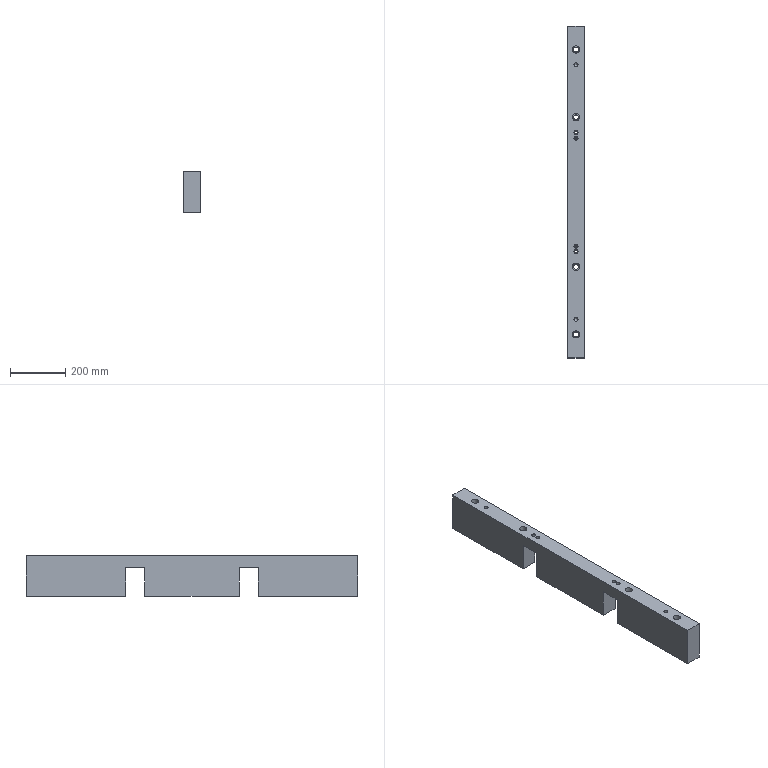Part | STEP file | lll_id2318_x_t | 1 solid | 42 faces | box 60 x 1200 x 147.5 mm | volume 9489564 mm3 | plane 22 | cylinder 18 | cone 2 | commonest cylinder face diameters 9.009 x4 14.508 x4 18.009 x4 26.008 x4 14.506 x2
STEP:
#1=CARTESIAN_POINT('',(2393.689,-215.498,370.));
#2=VERTEX_POINT('',#1);
#3=CARTESIAN_POINT('',(2386.435,-215.498,370.));
#4=DIRECTION('',(0.,0.,-1.));
#5=DIRECTION('',(1.,0.,0.));
#6=AXIS2_PLACEMENT_3D('',#3,#4,#5);
#7=CIRCLE('',#6,7.254);
#8=EDGE_CURVE('',#2,#2,#7,.T.);
#9=ORIENTED_EDGE('',*,*,#8,.T.);
#10=EDGE_LOOP('',(#9));
#11=FACE_BOUND('',#10,.T.);
#12=CARTESIAN_POINT('',(2393.689,-195.498,370.));
#13=VERTEX_POINT('',#12);
#14=CARTESIAN_POINT('',(2386.435,-195.498,370.));
#15=DIRECTION('',(0.,0.,-1.));
#16=DIRECTION('',(1.,0.,0.));
#17=AXIS2_PLACEMENT_3D('',#14,#15,#16);
#18=CIRCLE('',#17,7.254);
#19=EDGE_CURVE('',#13,#13,#18,.T.);
#20=ORIENTED_EDGE('',*,*,#19,.T.);
#21=EDGE_LOOP('',(#20));
#22=FACE_BOUND('',#21,.T.);
#23=CARTESIAN_POINT('',(2393.689,195.,370.));
#24=VERTEX_POINT('',#23);
#25=CARTESIAN_POINT('',(2386.435,195.,370.));
#26=DIRECTION('',(0.,0.,-1.));
#27=DIRECTION('',(1.,0.,0.));
#28=AXIS2_PLACEMENT_3D('',#25,#26,#27);
#29=CIRCLE('',#28,7.254);
#30=EDGE_CURVE('',#24,#24,#29,.T.);
#31=ORIENTED_EDGE('',*,*,#30,.T.);
#32=EDGE_LOOP('',(#31));
#33=FACE_BOUND('',#32,.T.);
#34=CARTESIAN_POINT('',(2393.689,215.,370.));
#35=VERTEX_POINT('',#34);
#36=CARTESIAN_POINT('',(2386.435,215.,370.));
#37=DIRECTION('',(0.,0.,-1.));
#38=DIRECTION('',(1.,0.,0.));
#39=AXIS2_PLACEMENT_3D('',#36,#37,#38);
#40=CIRCLE('',#39,7.254);
#41=EDGE_CURVE('',#35,#35,#40,.T.);
#42=ORIENTED_EDGE('',*,*,#41,.T.);
#43=EDGE_LOOP('',(#42));
#44=FACE_BOUND('',#43,.T.);
#45=CARTESIAN_POINT('',(2399.439,270.,370.));
#46=VERTEX_POINT('',#45);
#47=CARTESIAN_POINT('',(2386.435,270.,370.));
#48=DIRECTION('',(0.,0.,1.));
#49=DIRECTION('',(1.,0.,0.));
#50=AXIS2_PLACEMENT_3D('',#47,#48,#49);
#51=CIRCLE('',#50,13.004);
#52=EDGE_CURVE('',#46,#46,#51,.T.);
#53=ORIENTED_EDGE('',*,*,#52,.F.);
#54=EDGE_LOOP('',(#53));
#55=FACE_BOUND('',#54,.T.);
#56=CARTESIAN_POINT('',(2399.439,-270.,370.));
#57=VERTEX_POINT('',#56);
#58=CARTESIAN_POINT('',(2386.435,-270.,370.));
#59=DIRECTION('',(0.,0.,-1.));
#60=DIRECTION('',(1.,0.,0.));
#61=AXIS2_PLACEMENT_3D('',#58,#59,#60);
#62=CIRCLE('',#61,13.004);
#63=EDGE_CURVE('',#57,#57,#62,.T.);
#64=ORIENTED_EDGE('',*,*,#63,.T.);
#65=EDGE_LOOP('',(#64));
#66=FACE_BOUND('',#65,.T.);
#67=CARTESIAN_POINT('',(2399.439,-515.,370.));
#68=VERTEX_POINT('',#67);
#69=CARTESIAN_POINT('',(2386.435,-515.,370.));
#70=DIRECTION('',(0.,0.,-1.));
#71=DIRECTION('',(1.,0.,0.));
#72=AXIS2_PLACEMENT_3D('',#69,#70,#71);
#73=CIRCLE('',#72,13.004);
#74=EDGE_CURVE('',#68,#68,#73,.T.);
#75=ORIENTED_EDGE('',*,*,#74,.T.);
#76=EDGE_LOOP('',(#75));
#77=FACE_BOUND('',#76,.T.);
#78=CARTESIAN_POINT('',(2416.435,600.,370.));
#79=VERTEX_POINT('',#78);
#80=CARTESIAN_POINT('',(2356.435,600.,370.));
#81=VERTEX_POINT('',#80);
#82=CARTESIAN_POINT('',(6326.435,600.,370.));
#83=DIRECTION('',(-1.,0.,0.));
#84=VECTOR('',#83,1.);
#85=LINE('',#82,#84);
#86=EDGE_CURVE('',#79,#81,#85,.T.);
#87=ORIENTED_EDGE('',*,*,#86,.T.);
#88=CARTESIAN_POINT('',(2356.435,-600.,370.));
#89=VERTEX_POINT('',#88);
#90=CARTESIAN_POINT('',(2356.435,600.,370.));
#91=DIRECTION('',(0.,-1.,0.));
#92=VECTOR('',#91,1.);
#93=LINE('',#90,#92);
#94=EDGE_CURVE('',#81,#89,#93,.T.);
#95=ORIENTED_EDGE('',*,*,#94,.T.);
#96=CARTESIAN_POINT('',(2416.435,-600.,370.));
#97=VERTEX_POINT('',#96);
#98=CARTESIAN_POINT('',(2356.435,-600.,370.));
#99=DIRECTION('',(1.,0.,0.));
#100=VECTOR('',#99,1.);
#101=LINE('',#98,#100);
#102=EDGE_CURVE('',#89,#97,#101,.T.);
#103=ORIENTED_EDGE('',*,*,#102,.T.);
#104=CARTESIAN_POINT('',(2416.435,1.,370.));
#105=DIRECTION('',(0.,1.,0.));
#106=VECTOR('',#105,1.);
#107=LINE('',#104,#106);
#108=EDGE_CURVE('',#97,#79,#107,.T.);
#109=ORIENTED_EDGE('',*,*,#108,.T.);
#110=EDGE_LOOP('',(#87,#95,#103,#109));
#111=FACE_BOUND('',#110,.T.);
#112=CARTESIAN_POINT('',(2399.439,515.,370.));
#113=VERTEX_POINT('',#112);
#114=CARTESIAN_POINT('',(2386.435,515.,370.));
#115=DIRECTION('',(0.,0.,1.));
#116=DIRECTION('',(1.,0.,0.));
#117=AXIS2_PLACEMENT_3D('',#114,#115,#116);
#118=CIRCLE('',#117,13.004);
#119=EDGE_CURVE('',#113,#113,#118,.T.);
#120=ORIENTED_EDGE('',*,*,#119,.F.);
#121=EDGE_LOOP('',(#120));
#122=FACE_BOUND('',#121,.T.);
#123=CARTESIAN_POINT('',(2393.688,-460.,370.));
#124=VERTEX_POINT('',#123);
#125=CARTESIAN_POINT('',(2386.435,-460.,370.));
#126=DIRECTION('',(0.,0.,-1.));
#127=DIRECTION('',(1.,0.,0.));
#128=AXIS2_PLACEMENT_3D('',#125,#126,#127);
#129=CIRCLE('',#128,7.253);
#130=EDGE_CURVE('',#124,#124,#129,.T.);
#131=ORIENTED_EDGE('',*,*,#130,.T.);
#132=EDGE_LOOP('',(#131));
#133=FACE_BOUND('',#132,.T.);
#134=CARTESIAN_POINT('',(2393.688,460.,370.));
#135=VERTEX_POINT('',#134);
#136=CARTESIAN_POINT('',(2386.435,460.,370.));
#137=DIRECTION('',(0.,0.,1.));
#138=DIRECTION('',(1.,0.,0.));
#139=AXIS2_PLACEMENT_3D('',#136,#137,#138);
#140=CIRCLE('',#139,7.253);
#141=EDGE_CURVE('',#135,#135,#140,.T.);
#142=ORIENTED_EDGE('',*,*,#141,.F.);
#143=EDGE_LOOP('',(#142));
#144=FACE_BOUND('',#143,.T.);
#145=CARTESIAN_POINT('',(170.12,1.,370.));
#146=DIRECTION('',(0.,0.,-1.));
#147=DIRECTION('',(1.,0.,0.));
#148=AXIS2_PLACEMENT_3D('',#145,#146,#147);
#149=PLANE('',#148);
#150=ADVANCED_FACE('',(#11,#22,#33,#44,#55,#66,#77,#111,#122,#133,#144),#149,.F.);
#151=CARTESIAN_POINT('',(2416.435,170.249,222.5));
#152=VERTEX_POINT('',#151);
#153=CARTESIAN_POINT('',(2356.435,170.249,222.5));
#154=VERTEX_POINT('',#153);
#155=CARTESIAN_POINT('',(170.12,170.249,222.5));
#156=DIRECTION('',(-1.,0.,0.));
#157=VECTOR('',#156,1.);
#158=LINE('',#155,#157);
#159=EDGE_CURVE('',#152,#154,#158,.T.);
#160=ORIENTED_EDGE('',*,*,#159,.F.);
#161=CARTESIAN_POINT('',(2416.435,-170.249,222.5));
#162=VERTEX_POINT('',#161);
#163=CARTESIAN_POINT('',(2416.435,1.,222.5));
#164=DIRECTION('',(0.,-1.,0.));
#165=VECTOR('',#164,1.);
#166=LINE('',#163,#165);
#167=EDGE_CURVE('',#152,#162,#166,.T.);
#168=ORIENTED_EDGE('',*,*,#167,.T.);
#169=CARTESIAN_POINT('',(2356.435,-170.249,222.5));
#170=VERTEX_POINT('',#169);
#171=CARTESIAN_POINT('',(170.12,-170.249,222.5));
#172=DIRECTION('',(1.,0.,0.));
#173=VECTOR('',#172,1.);
#174=LINE('',#171,#173);
#175=EDGE_CURVE('',#170,#162,#174,.T.);
#176=ORIENTED_EDGE('',*,*,#175,.F.);
#177=CARTESIAN_POINT('',(2356.435,600.,222.5));
#178=DIRECTION('',(0.,-1.,0.));
#179=VECTOR('',#178,1.);
#180=LINE('',#177,#179);
#181=EDGE_CURVE('',#154,#170,#180,.T.);
#182=ORIENTED_EDGE('',*,*,#181,.F.);
#183=EDGE_LOOP('',(#160,#168,#176,#182));
#184=FACE_OUTER_BOUND('',#183,.T.);
#185=CARTESIAN_POINT('',(170.12,1.,222.5));
#186=DIRECTION('',(0.,0.,-1.));
#187=DIRECTION('',(1.,0.,0.));
#188=AXIS2_PLACEMENT_3D('',#185,#186,#187);
#189=PLANE('',#188);
#190=ADVANCED_FACE('',(#184),#189,.T.);
#191=CARTESIAN_POINT('',(2377.431,270.,222.5));
#192=VERTEX_POINT('',#191);
#193=CARTESIAN_POINT('',(2386.435,270.,222.5));
#194=DIRECTION('',(0.,0.,-1.));
#195=DIRECTION('',(-1.,0.,0.));
#196=AXIS2_PLACEMENT_3D('',#193,#194,#195);
#197=CIRCLE('',#196,9.005);
#198=EDGE_CURVE('',#192,#192,#197,.T.);
#199=ORIENTED_EDGE('',*,*,#198,.F.);
#200=EDGE_LOOP('',(#199));
#201=FACE_BOUND('',#200,.T.);
#202=CARTESIAN_POINT('',(2356.435,240.249,222.5));
#203=VERTEX_POINT('',#202);
#204=CARTESIAN_POINT('',(2416.435,240.249,222.5));
#205=VERTEX_POINT('',#204);
#206=CARTESIAN_POINT('',(170.12,240.249,222.5));
#207=DIRECTION('',(1.,0.,0.));
#208=VECTOR('',#207,1.);
#209=LINE('',#206,#208);
#210=EDGE_CURVE('',#203,#205,#209,.T.);
#211=ORIENTED_EDGE('',*,*,#210,.F.);
#212=CARTESIAN_POINT('',(2356.435,600.,222.5));
#213=VERTEX_POINT('',#212);
#214=CARTESIAN_POINT('',(2356.435,600.,222.5));
#215=DIRECTION('',(0.,-1.,0.));
#216=VECTOR('',#215,1.);
#217=LINE('',#214,#216);
#218=EDGE_CURVE('',#213,#203,#217,.T.);
#219=ORIENTED_EDGE('',*,*,#218,.F.);
#220=CARTESIAN_POINT('',(2416.435,600.,222.5));
#221=VERTEX_POINT('',#220);
#222=CARTESIAN_POINT('',(6326.435,600.,222.5));
#223=DIRECTION('',(-1.,0.,0.));
#224=VECTOR('',#223,1.);
#225=LINE('',#222,#224);
#226=EDGE_CURVE('',#221,#213,#225,.T.);
#227=ORIENTED_EDGE('',*,*,#226,.F.);
#228=CARTESIAN_POINT('',(2416.435,1.,222.5));
#229=DIRECTION('',(0.,-1.,0.));
#230=VECTOR('',#229,1.);
#231=LINE('',#228,#230);
#232=EDGE_CURVE('',#221,#205,#231,.T.);
#233=ORIENTED_EDGE('',*,*,#232,.T.);
#234=EDGE_LOOP('',(#211,#219,#227,#233));
#235=FACE_BOUND('',#234,.T.);
#236=CARTESIAN_POINT('',(2395.44,515.,222.5));
#237=VERTEX_POINT('',#236);
#238=CARTESIAN_POINT('',(2386.435,515.,222.5));
#239=DIRECTION('',(0.,0.,-1.));
#240=DIRECTION('',(1.,0.,0.));
#241=AXIS2_PLACEMENT_3D('',#238,#239,#240);
#242=CIRCLE('',#241,9.005);
#243=EDGE_CURVE('',#237,#237,#242,.T.);
#244=ORIENTED_EDGE('',*,*,#243,.F.);
#245=EDGE_LOOP('',(#244));
#246=FACE_BOUND('',#245,.T.);
#247=CARTESIAN_POINT('',(170.12,1.,222.5));
#248=DIRECTION('',(0.,0.,-1.));
#249=DIRECTION('',(1.,0.,0.));
#250=AXIS2_PLACEMENT_3D('',#247,#248,#249);
#251=PLANE('',#250);
#252=ADVANCED_FACE('',(#201,#235,#246),#251,.T.);
#253=CARTESIAN_POINT('',(2377.431,-270.,222.5));
#254=VERTEX_POINT('',#253);
#255=CARTESIAN_POINT('',(2386.435,-270.,222.5));
#256=DIRECTION('',(0.,0.,1.));
#257=DIRECTION('',(-1.,0.,0.));
#258=AXIS2_PLACEMENT_3D('',#255,#256,#257);
#259=CIRCLE('',#258,9.005);
#260=EDGE_CURVE('',#254,#254,#259,.T.);
#261=ORIENTED_EDGE('',*,*,#260,.T.);
#262=EDGE_LOOP('',(#261));
#263=FACE_BOUND('',#262,.T.);
#264=CARTESIAN_POINT('',(2416.435,-240.249,222.5));
#265=VERTEX_POINT('',#264);
#266=CARTESIAN_POINT('',(2356.435,-240.249,222.5));
#267=VERTEX_POINT('',#266);
#268=CARTESIAN_POINT('',(170.12,-240.249,222.5));
#269=DIRECTION('',(-1.,0.,0.));
#270=VECTOR('',#269,1.);
#271=LINE('',#268,#270);
#272=EDGE_CURVE('',#265,#267,#271,.T.);
#273=ORIENTED_EDGE('',*,*,#272,.F.);
#274=CARTESIAN_POINT('',(2416.435,-600.,222.5));
#275=VERTEX_POINT('',#274);
#276=CARTESIAN_POINT('',(2416.435,1.,222.5));
#277=DIRECTION('',(0.,-1.,0.));
#278=VECTOR('',#277,1.);
#279=LINE('',#276,#278);
#280=EDGE_CURVE('',#265,#275,#279,.T.);
#281=ORIENTED_EDGE('',*,*,#280,.T.);
#282=CARTESIAN_POINT('',(2356.435,-600.,222.5));
#283=VERTEX_POINT('',#282);
#284=CARTESIAN_POINT('',(2356.435,-600.,222.5));
#285=DIRECTION('',(1.,0.,0.));
#286=VECTOR('',#285,1.);
#287=LINE('',#284,#286);
#288=EDGE_CURVE('',#283,#275,#287,.T.);
#289=ORIENTED_EDGE('',*,*,#288,.F.);
#290=CARTESIAN_POINT('',(2356.435,600.,222.5));
#291=DIRECTION('',(0.,-1.,0.));
#292=VECTOR('',#291,1.);
#293=LINE('',#290,#292);
#294=EDGE_CURVE('',#267,#283,#293,.T.);
#295=ORIENTED_EDGE('',*,*,#294,.F.);
#296=EDGE_LOOP('',(#273,#281,#289,#295));
#297=FACE_BOUND('',#296,.T.);
#298=CARTESIAN_POINT('',(2395.44,-515.,222.5));
#299=VERTEX_POINT('',#298);
#300=CARTESIAN_POINT('',(2386.435,-515.,222.5));
#301=DIRECTION('',(0.,0.,1.));
#302=DIRECTION('',(1.,0.,0.));
#303=AXIS2_PLACEMENT_3D('',#300,#301,#302);
#304=CIRCLE('',#303,9.005);
#305=EDGE_CURVE('',#299,#299,#304,.T.);
#306=ORIENTED_EDGE('',*,*,#305,.T.);
#307=EDGE_LOOP('',(#306));
#308=FACE_BOUND('',#307,.T.);
#309=CARTESIAN_POINT('',(170.12,1.,222.5));
#310=DIRECTION('',(0.,0.,-1.));
#311=DIRECTION('',(1.,0.,0.));
#312=AXIS2_PLACEMENT_3D('',#309,#310,#311);
#313=PLANE('',#312);
#314=ADVANCED_FACE('',(#263,#297,#308),#313,.T.);
#315=CARTESIAN_POINT('',(2356.435,-170.249,326.5));
#316=VERTEX_POINT('',#315);
#317=CARTESIAN_POINT('',(2356.435,-240.249,326.5));
#318=VERTEX_POINT('',#317);
#319=CARTESIAN_POINT('',(2356.435,44.502,326.5));
#320=DIRECTION('',(0.,-1.,0.));
#321=VECTOR('',#320,1.);
#322=LINE('',#319,#321);
#323=EDGE_CURVE('',#316,#318,#322,.T.);
#324=ORIENTED_EDGE('',*,*,#323,.T.);
#325=CARTESIAN_POINT('',(2356.435,-240.249,363.5));
#326=DIRECTION('',(0.,0.,1.));
#327=VECTOR('',#326,1.);
#328=LINE('',#325,#327);
#329=EDGE_CURVE('',#267,#318,#328,.T.);
#330=ORIENTED_EDGE('',*,*,#329,.F.);
#331=ORIENTED_EDGE('',*,*,#294,.T.);
#332=CARTESIAN_POINT('',(2356.435,-600.,310.));
#333=DIRECTION('',(0.,0.,-1.));
#334=VECTOR('',#333,1.);
#335=LINE('',#332,#334);
#336=EDGE_CURVE('',#89,#283,#335,.T.);
#337=ORIENTED_EDGE('',*,*,#336,.F.);
#338=ORIENTED_EDGE('',*,*,#94,.F.);
#339=CARTESIAN_POINT('',(2356.435,600.,310.));
#340=DIRECTION('',(0.,0.,-1.));
#341=VECTOR('',#340,1.);
#342=LINE('',#339,#341);
#343=EDGE_CURVE('',#81,#213,#342,.T.);
#344=ORIENTED_EDGE('',*,*,#343,.T.);
#345=ORIENTED_EDGE('',*,*,#218,.T.);
#346=CARTESIAN_POINT('',(2356.435,240.249,326.5));
#347=VERTEX_POINT('',#346);
#348=CARTESIAN_POINT('',(2356.435,240.249,363.5));
#349=DIRECTION('',(0.,0.,-1.));
#350=VECTOR('',#349,1.);
#351=LINE('',#348,#350);
#352=EDGE_CURVE('',#347,#203,#351,.T.);
#353=ORIENTED_EDGE('',*,*,#352,.F.);
#354=CARTESIAN_POINT('',(2356.435,170.249,326.5));
#355=VERTEX_POINT('',#354);
#356=CARTESIAN_POINT('',(2356.435,455.,326.5));
#357=DIRECTION('',(0.,-1.,0.));
#358=VECTOR('',#357,1.);
#359=LINE('',#356,#358);
#360=EDGE_CURVE('',#347,#355,#359,.T.);
#361=ORIENTED_EDGE('',*,*,#360,.T.);
#362=CARTESIAN_POINT('',(2356.435,170.249,363.5));
#363=DIRECTION('',(0.,0.,1.));
#364=VECTOR('',#363,1.);
#365=LINE('',#362,#364);
#366=EDGE_CURVE('',#154,#355,#365,.T.);
#367=ORIENTED_EDGE('',*,*,#366,.F.);
#368=ORIENTED_EDGE('',*,*,#181,.T.);
#369=CARTESIAN_POINT('',(2356.435,-170.249,363.5));
#370=DIRECTION('',(0.,0.,-1.));
#371=VECTOR('',#370,1.);
#372=LINE('',#369,#371);
#373=EDGE_CURVE('',#316,#170,#372,.T.);
#374=ORIENTED_EDGE('',*,*,#373,.F.);
#375=EDGE_LOOP('',(#324,#330,#331,#337,#338,#344,#345,#353,#361,#367,#368,#374));
#376=FACE_OUTER_BOUND('',#375,.T.);
#377=CARTESIAN_POINT('',(2356.435,600.,310.));
#378=DIRECTION('',(-1.,0.,0.));
#379=DIRECTION('',(0.,0.,-1.));
#380=AXIS2_PLACEMENT_3D('',#377,#378,#379);
#381=PLANE('',#380);
#382=ADVANCED_FACE('',(#376),#381,.T.);
#383=CARTESIAN_POINT('',(2416.435,-600.,310.));
#384=DIRECTION('',(0.,0.,-1.));
#385=VECTOR('',#384,1.);
#386=LINE('',#383,#385);
#387=EDGE_CURVE('',#97,#275,#386,.T.);
#388=ORIENTED_EDGE('',*,*,#387,.F.);
#389=ORIENTED_EDGE('',*,*,#102,.F.);
#390=ORIENTED_EDGE('',*,*,#336,.T.);
#391=ORIENTED_EDGE('',*,*,#288,.T.);
#392=EDGE_LOOP('',(#388,#389,#390,#391));
#393=FACE_OUTER_BOUND('',#392,.T.);
#394=CARTESIAN_POINT('',(2356.435,-600.,310.));
#395=DIRECTION('',(0.,-1.,0.));
#396=DIRECTION('',(0.,0.,-1.));
#397=AXIS2_PLACEMENT_3D('',#394,#395,#396);
#398=PLANE('',#397);
#399=ADVANCED_FACE('',(#393),#398,.T.);
#400=CARTESIAN_POINT('',(2416.435,600.,310.));
#401=DIRECTION('',(0.,0.,1.));
#402=VECTOR('',#401,1.);
#403=LINE('',#400,#402);
#404=EDGE_CURVE('',#221,#79,#403,.T.);
#405=ORIENTED_EDGE('',*,*,#404,.F.);
#406=ORIENTED_EDGE('',*,*,#226,.T.);
#407=ORIENTED_EDGE('',*,*,#343,.F.);
#408=ORIENTED_EDGE('',*,*,#86,.F.);
#409=EDGE_LOOP('',(#405,#406,#407,#408));
#410=FACE_OUTER_BOUND('',#409,.T.);
#411=CARTESIAN_POINT('',(6326.435,600.,310.));
#412=DIRECTION('',(0.,1.,0.));
#413=DIRECTION('',(0.,0.,1.));
#414=AXIS2_PLACEMENT_3D('',#411,#412,#413);
#415=PLANE('',#414);
#416=ADVANCED_FACE('',(#410),#415,.T.);
#417=CARTESIAN_POINT('',(2416.435,-240.249,326.5));
#418=VERTEX_POINT('',#417);
#419=CARTESIAN_POINT('',(2416.435,-240.249,294.75));
#420=DIRECTION('',(0.,0.,1.));
#421=VECTOR('',#420,1.);
#422=LINE('',#419,#421);
#423=EDGE_CURVE('',#265,#418,#422,.T.);
#424=ORIENTED_EDGE('',*,*,#423,.T.);
#425=CARTESIAN_POINT('',(2416.435,-170.249,326.5));
#426=VERTEX_POINT('',#425);
#427=CARTESIAN_POINT('',(2416.435,-555.498,326.5));
#428=DIRECTION('',(0.,-1.,0.));
#429=VECTOR('',#428,1.);
#430=LINE('',#427,#429);
#431=EDGE_CURVE('',#426,#418,#430,.T.);
#432=ORIENTED_EDGE('',*,*,#431,.F.);
#433=CARTESIAN_POINT('',(2416.435,-170.249,294.75));
#434=DIRECTION('',(0.,0.,-1.));
#435=VECTOR('',#434,1.);
#436=LINE('',#433,#435);
#437=EDGE_CURVE('',#426,#162,#436,.T.);
#438=ORIENTED_EDGE('',*,*,#437,.T.);
#439=ORIENTED_EDGE('',*,*,#167,.F.);
#440=CARTESIAN_POINT('',(2416.435,170.249,326.5));
#441=VERTEX_POINT('',#440);
#442=CARTESIAN_POINT('',(2416.435,170.249,294.75));
#443=DIRECTION('',(0.,0.,1.));
#444=VECTOR('',#443,1.);
#445=LINE('',#442,#444);
#446=EDGE_CURVE('',#152,#441,#445,.T.);
#447=ORIENTED_EDGE('',*,*,#446,.T.);
#448=CARTESIAN_POINT('',(2416.435,240.249,326.5));
#449=VERTEX_POINT('',#448);
#450=CARTESIAN_POINT('',(2416.435,-145.,326.5));
#451=DIRECTION('',(0.,-1.,0.));
#452=VECTOR('',#451,1.);
#453=LINE('',#450,#452);
#454=EDGE_CURVE('',#449,#441,#453,.T.);
#455=ORIENTED_EDGE('',*,*,#454,.F.);
#456=CARTESIAN_POINT('',(2416.435,240.249,294.75));
#457=DIRECTION('',(0.,0.,-1.));
#458=VECTOR('',#457,1.);
#459=LINE('',#456,#458);
#460=EDGE_CURVE('',#449,#205,#459,.T.);
#461=ORIENTED_EDGE('',*,*,#460,.T.);
#462=ORIENTED_EDGE('',*,*,#232,.F.);
#463=ORIENTED_EDGE('',*,*,#404,.T.);
#464=ORIENTED_EDGE('',*,*,#108,.F.);
#465=ORIENTED_EDGE('',*,*,#387,.T.);
#466=ORIENTED_EDGE('',*,*,#280,.F.);
#467=EDGE_LOOP('',(#424,#432,#438,#439,#447,#455,#461,#462,#463,#464,#465,#466));
#468=FACE_OUTER_BOUND('',#467,.T.);
#469=CARTESIAN_POINT('',(2416.435,0.,241.25));
#470=DIRECTION('',(-1.,0.,0.));
#471=DIRECTION('',(0.,0.,-1.));
#472=AXIS2_PLACEMENT_3D('',#469,#470,#471);
#473=PLANE('',#472);
#474=ADVANCED_FACE('',(#468),#473,.F.);
#475=CARTESIAN_POINT('',(2377.431,-515.,302.5));
#476=VERTEX_POINT('',#475);
#477=CARTESIAN_POINT('',(2386.435,-515.,302.5));
#478=DIRECTION('',(0.,0.,-1.));
#479=DIRECTION('',(-1.,0.,0.));
#480=AXIS2_PLACEMENT_3D('',#477,#478,#479);
#481=CIRCLE('',#480,9.005);
#482=EDGE_CURVE('',#476,#476,#481,.T.);
#483=ORIENTED_EDGE('',*,*,#482,.F.);
#484=EDGE_LOOP('',(#483));
#485=FACE_BOUND('',#484,.T.);
#486=ORIENTED_EDGE('',*,*,#305,.F.);
#487=EDGE_LOOP('',(#486));
#488=FACE_BOUND('',#487,.T.);
#489=CARTESIAN_POINT('',(2386.435,-515.,420.));
#490=DIRECTION('',(0.,0.,-1.));
#491=DIRECTION('',(1.,0.,0.));
#492=AXIS2_PLACEMENT_3D('',#489,#490,#491);
#493=CYLINDRICAL_SURFACE('',#492,9.005);
#494=ADVANCED_FACE('',(#485,#488),#493,.F.);
#495=ORIENTED_EDGE('',*,*,#482,.T.);
#496=EDGE_LOOP('',(#495));
#497=FACE_BOUND('',#496,.T.);
#498=CARTESIAN_POINT('',(2399.439,-515.,302.5));
#499=VERTEX_POINT('',#498);
#500=CARTESIAN_POINT('',(2386.435,-515.,302.5));
#501=DIRECTION('',(0.,0.,-1.));
#502=DIRECTION('',(-1.,0.,0.));
#503=AXIS2_PLACEMENT_3D('',#500,#501,#502);
#504=CIRCLE('',#503,13.004);
#505=EDGE_CURVE('',#499,#499,#504,.T.);
#506=ORIENTED_EDGE('',*,*,#505,.F.);
#507=EDGE_LOOP('',(#506));
#508=FACE_BOUND('',#507,.T.);
#509=CARTESIAN_POINT('',(2386.435,-515.,302.5));
#510=DIRECTION('',(0.,0.,-1.));
#511=DIRECTION('',(-1.,0.,0.));
#512=AXIS2_PLACEMENT_3D('',#509,#510,#511);
#513=PLANE('',#512);
#514=ADVANCED_FACE('',(#497,#508),#513,.F.);
#515=ORIENTED_EDGE('',*,*,#505,.T.);
#516=EDGE_LOOP('',(#515));
#517=FACE_BOUND('',#516,.T.);
#518=ORIENTED_EDGE('',*,*,#74,.F.);
#519=EDGE_LOOP('',(#518));
#520=FACE_BOUND('',#519,.T.);
#521=CARTESIAN_POINT('',(2386.435,-515.,370.));
#522=DIRECTION('',(0.,0.,-1.));
#523=DIRECTION('',(1.,0.,0.));
#524=AXIS2_PLACEMENT_3D('',#521,#522,#523);
#525=CYLINDRICAL_SURFACE('',#524,13.004);
#526=ADVANCED_FACE('',(#517,#520),#525,.F.);
#527=CARTESIAN_POINT('',(2377.431,-270.,302.5));
#528=VERTEX_POINT('',#527);
#529=CARTESIAN_POINT('',(2386.435,-270.,302.5));
#530=DIRECTION('',(0.,0.,-1.));
#531=DIRECTION('',(-1.,0.,0.));
#532=AXIS2_PLACEMENT_3D('',#529,#530,#531);
#533=CIRCLE('',#532,9.005);
#534=EDGE_CURVE('',#528,#528,#533,.T.);
#535=ORIENTED_EDGE('',*,*,#534,.F.);
#536=EDGE_LOOP('',(#535));
#537=FACE_BOUND('',#536,.T.);
#538=ORIENTED_EDGE('',*,*,#260,.F.);
#539=EDGE_LOOP('',(#538));
#540=FACE_BOUND('',#539,.T.);
#541=CARTESIAN_POINT('',(2386.435,-270.,420.));
#542=DIRECTION('',(0.,0.,-1.));
#543=DIRECTION('',(1.,0.,0.));
#544=AXIS2_PLACEMENT_3D('',#541,#542,#543);
#545=CYLINDRICAL_SURFACE('',#544,9.005);
#546=ADVANCED_FACE('',(#537,#540),#545,.F.);
#547=ORIENTED_EDGE('',*,*,#534,.T.);
#548=EDGE_LOOP('',(#547));
#549=FACE_BOUND('',#548,.T.);
#550=CARTESIAN_POINT('',(2399.439,-270.,302.5));
#551=VERTEX_POINT('',#550);
#552=CARTESIAN_POINT('',(2386.435,-270.,302.5));
#553=DIRECTION('',(0.,0.,-1.));
#554=DIRECTION('',(1.,0.,0.));
#555=AXIS2_PLACEMENT_3D('',#552,#553,#554);
#556=CIRCLE('',#555,13.004);
#557=EDGE_CURVE('',#551,#551,#556,.T.);
#558=ORIENTED_EDGE('',*,*,#557,.F.);
#559=EDGE_LOOP('',(#558));
#560=FACE_BOUND('',#559,.T.);
#561=CARTESIAN_POINT('',(2386.435,-270.,302.5));
#562=DIRECTION('',(0.,0.,-1.));
#563=DIRECTION('',(-1.,0.,0.));
#564=AXIS2_PLACEMENT_3D('',#561,#562,#563);
#565=PLANE('',#564);
#566=ADVANCED_FACE('',(#549,#560),#565,.F.);
#567=ORIENTED_EDGE('',*,*,#557,.T.);
#568=EDGE_LOOP('',(#567));
#569=FACE_BOUND('',#568,.T.);
#570=ORIENTED_EDGE('',*,*,#63,.F.);
#571=EDGE_LOOP('',(#570));
#572=FACE_BOUND('',#571,.T.);
#573=CARTESIAN_POINT('',(2386.435,-270.,370.));
#574=DIRECTION('',(0.,0.,-1.));
#575=DIRECTION('',(1.,0.,0.));
#576=AXIS2_PLACEMENT_3D('',#573,#574,#575);
#577=CYLINDRICAL_SURFACE('',#576,13.004);
#578=ADVANCED_FACE('',(#569,#572),#577,.F.);
#579=CARTESIAN_POINT('',(2377.431,270.,302.5));
#580=VERTEX_POINT('',#579);
#581=CARTESIAN_POINT('',(2386.435,270.,302.5));
#582=DIRECTION('',(0.,0.,1.));
#583=DIRECTION('',(-1.,0.,0.));
#584=AXIS2_PLACEMENT_3D('',#581,#582,#583);
#585=CIRCLE('',#584,9.005);
#586=EDGE_CURVE('',#580,#580,#585,.T.);
#587=ORIENTED_EDGE('',*,*,#586,.T.);
#588=EDGE_LOOP('',(#587));
#589=FACE_BOUND('',#588,.T.);
#590=ORIENTED_EDGE('',*,*,#198,.T.);
#591=EDGE_LOOP('',(#590));
#592=FACE_BOUND('',#591,.T.);
#593=CARTESIAN_POINT('',(2386.435,270.,420.));
#594=DIRECTION('',(0.,0.,-1.));
#595=DIRECTION('',(1.,0.,0.));
#596=AXIS2_PLACEMENT_3D('',#593,#594,#595);
#597=CYLINDRICAL_SURFACE('',#596,9.005);
#598=ADVANCED_FACE('',(#589,#592),#597,.F.);
#599=ORIENTED_EDGE('',*,*,#586,.F.);
#600=EDGE_LOOP('',(#599));
#601=FACE_BOUND('',#600,.T.);
#602=CARTESIAN_POINT('',(2399.439,270.,302.5));
#603=VERTEX_POINT('',#602);
#604=CARTESIAN_POINT('',(2386.435,270.,302.5));
#605=DIRECTION('',(0.,0.,1.));
#606=DIRECTION('',(1.,0.,0.));
#607=AXIS2_PLACEMENT_3D('',#604,#605,#606);
#608=CIRCLE('',#607,13.004);
#609=EDGE_CURVE('',#603,#603,#608,.T.);
#610=ORIENTED_EDGE('',*,*,#609,.T.);
#611=EDGE_LOOP('',(#610));
#612=FACE_BOUND('',#611,.T.);
#613=CARTESIAN_POINT('',(2386.435,270.,302.5));
#614=DIRECTION('',(0.,0.,-1.));
#615=DIRECTION('',(-1.,0.,0.));
#616=AXIS2_PLACEMENT_3D('',#613,#614,#615);
#617=PLANE('',#616);
#618=ADVANCED_FACE('',(#601,#612),#617,.F.);
#619=ORIENTED_EDGE('',*,*,#609,.F.);
#620=EDGE_LOOP('',(#619));
#621=FACE_BOUND('',#620,.T.);
#622=ORIENTED_EDGE('',*,*,#52,.T.);
#623=EDGE_LOOP('',(#622));
#624=FACE_BOUND('',#623,.T.);
#625=CARTESIAN_POINT('',(2386.435,270.,370.));
#626=DIRECTION('',(0.,0.,-1.));
#627=DIRECTION('',(1.,0.,0.));
#628=AXIS2_PLACEMENT_3D('',#625,#626,#627);
#629=CYLINDRICAL_SURFACE('',#628,13.004);
#630=ADVANCED_FACE('',(#621,#624),#629,.F.);
#631=CARTESIAN_POINT('',(2377.431,515.,302.5));
#632=VERTEX_POINT('',#631);
#633=CARTESIAN_POINT('',(2386.435,515.,302.5));
#634=DIRECTION('',(0.,0.,1.));
#635=DIRECTION('',(-1.,0.,0.));
#636=AXIS2_PLACEMENT_3D('',#633,#634,#635);
#637=CIRCLE('',#636,9.005);
#638=EDGE_CURVE('',#632,#632,#637,.T.);
#639=ORIENTED_EDGE('',*,*,#638,.T.);
#640=EDGE_LOOP('',(#639));
#641=FACE_BOUND('',#640,.T.);
#642=ORIENTED_EDGE('',*,*,#243,.T.);
#643=EDGE_LOOP('',(#642));
#644=FACE_BOUND('',#643,.T.);
#645=CARTESIAN_POINT('',(2386.435,515.,420.));
#646=DIRECTION('',(0.,0.,-1.));
#647=DIRECTION('',(1.,0.,0.));
#648=AXIS2_PLACEMENT_3D('',#645,#646,#647);
#649=CYLINDRICAL_SURFACE('',#648,9.005);
#650=ADVANCED_FACE('',(#641,#644),#649,.F.);
#651=ORIENTED_EDGE('',*,*,#638,.F.);
#652=EDGE_LOOP('',(#651));
#653=FACE_BOUND('',#652,.T.);
#654=CARTESIAN_POINT('',(2399.439,515.,302.5));
#655=VERTEX_POINT('',#654);
#656=CARTESIAN_POINT('',(2386.435,515.,302.5));
#657=DIRECTION('',(0.,0.,1.));
#658=DIRECTION('',(1.,0.,0.));
#659=AXIS2_PLACEMENT_3D('',#656,#657,#658);
#660=CIRCLE('',#659,13.004);
#661=EDGE_CURVE('',#655,#655,#660,.T.);
#662=ORIENTED_EDGE('',*,*,#661,.T.);
#663=EDGE_LOOP('',(#662));
#664=FACE_BOUND('',#663,.T.);
#665=CARTESIAN_POINT('',(2386.435,515.,302.5));
#666=DIRECTION('',(0.,0.,-1.));
#667=DIRECTION('',(-1.,0.,0.));
#668=AXIS2_PLACEMENT_3D('',#665,#666,#667);
#669=PLANE('',#668);
#670=ADVANCED_FACE('',(#653,#664),#669,.F.);
#671=ORIENTED_EDGE('',*,*,#661,.F.);
#672=EDGE_LOOP('',(#671));
#673=FACE_BOUND('',#672,.T.);
#674=ORIENTED_EDGE('',*,*,#119,.T.);
#675=EDGE_LOOP('',(#674));
#676=FACE_BOUND('',#675,.T.);
#677=CARTESIAN_POINT('',(2386.435,515.,370.));
#678=DIRECTION('',(0.,0.,-1.));
#679=DIRECTION('',(1.,0.,0.));
#680=AXIS2_PLACEMENT_3D('',#677,#678,#679);
#681=CYLINDRICAL_SURFACE('',#680,13.004);
#682=ADVANCED_FACE('',(#673,#676),#681,.F.);
#683=ORIENTED_EDGE('',*,*,#373,.T.);
#684=ORIENTED_EDGE('',*,*,#175,.T.);
#685=ORIENTED_EDGE('',*,*,#437,.F.);
#686=CARTESIAN_POINT('',(2386.435,-170.249,326.5));
#687=DIRECTION('',(-1.,0.,0.));
#688=VECTOR('',#687,1.);
#689=LINE('',#686,#688);
#690=EDGE_CURVE('',#426,#316,#689,.T.);
#691=ORIENTED_EDGE('',*,*,#690,.T.);
#692=EDGE_LOOP('',(#683,#684,#685,#691));
#693=FACE_OUTER_BOUND('',#692,.T.);
#694=CARTESIAN_POINT('',(2386.435,-170.249,130.));
#695=DIRECTION('',(0.,1.,0.));
#696=DIRECTION('',(0.,0.,-1.));
#697=AXIS2_PLACEMENT_3D('',#694,#695,#696);
#698=PLANE('',#697);
#699=ADVANCED_FACE('',(#693),#698,.F.);
#700=ORIENTED_EDGE('',*,*,#329,.T.);
#701=CARTESIAN_POINT('',(2386.435,-240.249,326.5));
#702=DIRECTION('',(1.,0.,0.));
#703=VECTOR('',#702,1.);
#704=LINE('',#701,#703);
#705=EDGE_CURVE('',#318,#418,#704,.T.);
#706=ORIENTED_EDGE('',*,*,#705,.T.);
#707=ORIENTED_EDGE('',*,*,#423,.F.);
#708=ORIENTED_EDGE('',*,*,#272,.T.);
#709=EDGE_LOOP('',(#700,#706,#707,#708));
#710=FACE_OUTER_BOUND('',#709,.T.);
#711=CARTESIAN_POINT('',(2386.435,-240.249,130.));
#712=DIRECTION('',(0.,-1.,0.));
#713=DIRECTION('',(0.,0.,1.));
#714=AXIS2_PLACEMENT_3D('',#711,#712,#713);
#715=PLANE('',#714);
#716=ADVANCED_FACE('',(#710),#715,.F.);
#717=ORIENTED_EDGE('',*,*,#366,.T.);
#718=CARTESIAN_POINT('',(2386.435,170.249,326.5));
#719=DIRECTION('',(1.,0.,0.));
#720=VECTOR('',#719,1.);
#721=LINE('',#718,#720);
#722=EDGE_CURVE('',#355,#441,#721,.T.);
#723=ORIENTED_EDGE('',*,*,#722,.T.);
#724=ORIENTED_EDGE('',*,*,#446,.F.);
#725=ORIENTED_EDGE('',*,*,#159,.T.);
#726=EDGE_LOOP('',(#717,#723,#724,#725));
#727=FACE_OUTER_BOUND('',#726,.T.);
#728=CARTESIAN_POINT('',(2386.435,170.249,130.));
#729=DIRECTION('',(0.,-1.,0.));
#730=DIRECTION('',(0.,0.,-1.));
#731=AXIS2_PLACEMENT_3D('',#728,#729,#730);
#732=PLANE('',#731);
#733=ADVANCED_FACE('',(#727),#732,.F.);
#734=ORIENTED_EDGE('',*,*,#352,.T.);
#735=ORIENTED_EDGE('',*,*,#210,.T.);
#736=ORIENTED_EDGE('',*,*,#460,.F.);
#737=CARTESIAN_POINT('',(2386.435,240.249,326.5));
#738=DIRECTION('',(-1.,0.,0.));
#739=VECTOR('',#738,1.);
#740=LINE('',#737,#739);
#741=EDGE_CURVE('',#449,#347,#740,.T.);
#742=ORIENTED_EDGE('',*,*,#741,.T.);
#743=EDGE_LOOP('',(#734,#735,#736,#742));
#744=FACE_OUTER_BOUND('',#743,.T.);
#745=CARTESIAN_POINT('',(2386.435,240.249,130.));
#746=DIRECTION('',(0.,1.,0.));
#747=DIRECTION('',(0.,0.,1.));
#748=AXIS2_PLACEMENT_3D('',#745,#746,#747);
#749=PLANE('',#748);
#750=ADVANCED_FACE('',(#744),#749,.F.);
#751=CARTESIAN_POINT('',(2393.689,195.,351.5));
#752=VERTEX_POINT('',#751);
#753=CARTESIAN_POINT('',(2386.435,195.,351.5));
#754=DIRECTION('',(0.,0.,-1.));
#755=DIRECTION('',(1.,0.,0.));
#756=AXIS2_PLACEMENT_3D('',#753,#754,#755);
#757=CIRCLE('',#756,7.254);
#758=EDGE_CURVE('',#752,#752,#757,.T.);
#759=ORIENTED_EDGE('',*,*,#758,.T.);
#760=EDGE_LOOP('',(#759));
#761=FACE_BOUND('',#760,.T.);
#762=ORIENTED_EDGE('',*,*,#30,.F.);
#763=EDGE_LOOP('',(#762));
#764=FACE_BOUND('',#763,.T.);
#765=CARTESIAN_POINT('',(2386.435,195.,370.));
#766=DIRECTION('',(0.,0.,-1.));
#767=DIRECTION('',(1.,0.,0.));
#768=AXIS2_PLACEMENT_3D('',#765,#766,#767);
#769=CYLINDRICAL_SURFACE('',#768,7.254);
#770=ADVANCED_FACE('',(#761,#764),#769,.F.);
#771=CARTESIAN_POINT('',(2393.689,215.,351.5));
#772=VERTEX_POINT('',#771);
#773=CARTESIAN_POINT('',(2386.435,215.,351.5));
#774=DIRECTION('',(0.,0.,-1.));
#775=DIRECTION('',(1.,0.,0.));
#776=AXIS2_PLACEMENT_3D('',#773,#774,#775);
#777=CIRCLE('',#776,7.254);
#778=EDGE_CURVE('',#772,#772,#777,.T.);
#779=ORIENTED_EDGE('',*,*,#778,.T.);
#780=EDGE_LOOP('',(#779));
#781=FACE_BOUND('',#780,.T.);
#782=ORIENTED_EDGE('',*,*,#41,.F.);
#783=EDGE_LOOP('',(#782));
#784=FACE_BOUND('',#783,.T.);
#785=CARTESIAN_POINT('',(2386.435,215.,370.));
#786=DIRECTION('',(0.,0.,-1.));
#787=DIRECTION('',(1.,0.,0.));
#788=AXIS2_PLACEMENT_3D('',#785,#786,#787);
#789=CYLINDRICAL_SURFACE('',#788,7.254);
#790=ADVANCED_FACE('',(#781,#784),#789,.F.);
#791=CARTESIAN_POINT('',(2381.931,215.,351.5));
#792=VERTEX_POINT('',#791);
#793=CARTESIAN_POINT('',(2386.435,215.,351.5));
#794=DIRECTION('',(0.,0.,-1.));
#795=DIRECTION('',(-1.,0.,0.));
#796=AXIS2_PLACEMENT_3D('',#793,#794,#795);
#797=CIRCLE('',#796,4.505);
#798=EDGE_CURVE('',#792,#792,#797,.T.);
#799=ORIENTED_EDGE('',*,*,#798,.T.);
#800=EDGE_LOOP('',(#799));
#801=FACE_BOUND('',#800,.T.);
#802=ORIENTED_EDGE('',*,*,#778,.F.);
#803=EDGE_LOOP('',(#802));
#804=FACE_BOUND('',#803,.T.);
#805=CARTESIAN_POINT('',(2386.435,215.,351.5));
#806=DIRECTION('',(0.,0.,-1.));
#807=DIRECTION('',(-1.,0.,0.));
#808=AXIS2_PLACEMENT_3D('',#805,#806,#807);
#809=PLANE('',#808);
#810=ADVANCED_FACE('',(#801,#804),#809,.F.);
#811=CARTESIAN_POINT('',(2381.931,195.,351.5));
#812=VERTEX_POINT('',#811);
#813=CARTESIAN_POINT('',(2386.435,195.,351.5));
#814=DIRECTION('',(0.,0.,-1.));
#815=DIRECTION('',(-1.,0.,0.));
#816=AXIS2_PLACEMENT_3D('',#813,#814,#815);
#817=CIRCLE('',#816,4.505);
#818=EDGE_CURVE('',#812,#812,#817,.T.);
#819=ORIENTED_EDGE('',*,*,#818,.F.);
#820=EDGE_LOOP('',(#819));
#821=FACE_BOUND('',#820,.T.);
#822=CARTESIAN_POINT('',(2390.94,195.,326.5));
#823=VERTEX_POINT('',#822);
#824=CARTESIAN_POINT('',(2386.435,195.,326.5));
#825=DIRECTION('',(0.,0.,1.));
#826=DIRECTION('',(1.,0.,0.));
#827=AXIS2_PLACEMENT_3D('',#824,#825,#826);
#828=CIRCLE('',#827,4.505);
#829=EDGE_CURVE('',#823,#823,#828,.T.);
#830=ORIENTED_EDGE('',*,*,#829,.F.);
#831=EDGE_LOOP('',(#830));
#832=FACE_BOUND('',#831,.T.);
#833=CARTESIAN_POINT('',(2386.435,195.,370.));
#834=DIRECTION('',(0.,0.,-1.));
#835=DIRECTION('',(1.,0.,0.));
#836=AXIS2_PLACEMENT_3D('',#833,#834,#835);
#837=CYLINDRICAL_SURFACE('',#836,4.505);
#838=ADVANCED_FACE('',(#821,#832),#837,.F.);
#839=ORIENTED_EDGE('',*,*,#818,.T.);
#840=EDGE_LOOP('',(#839));
#841=FACE_BOUND('',#840,.T.);
#842=ORIENTED_EDGE('',*,*,#758,.F.);
#843=EDGE_LOOP('',(#842));
#844=FACE_BOUND('',#843,.T.);
#845=CARTESIAN_POINT('',(2386.435,195.,351.5));
#846=DIRECTION('',(0.,0.,-1.));
#847=DIRECTION('',(-1.,0.,0.));
#848=AXIS2_PLACEMENT_3D('',#845,#846,#847);
#849=PLANE('',#848);
#850=ADVANCED_FACE('',(#841,#844),#849,.F.);
#851=ORIENTED_EDGE('',*,*,#829,.T.);
#852=EDGE_LOOP('',(#851));
#853=FACE_BOUND('',#852,.T.);
#854=CARTESIAN_POINT('',(2390.94,215.,326.5));
#855=VERTEX_POINT('',#854);
#856=CARTESIAN_POINT('',(2386.435,215.,326.5));
#857=DIRECTION('',(0.,0.,1.));
#858=DIRECTION('',(1.,0.,0.));
#859=AXIS2_PLACEMENT_3D('',#856,#857,#858);
#860=CIRCLE('',#859,4.505);
#861=EDGE_CURVE('',#855,#855,#860,.T.);
#862=ORIENTED_EDGE('',*,*,#861,.T.);
#863=EDGE_LOOP('',(#862));
#864=FACE_BOUND('',#863,.T.);
#865=ORIENTED_EDGE('',*,*,#360,.F.);
#866=ORIENTED_EDGE('',*,*,#741,.F.);
#867=ORIENTED_EDGE('',*,*,#454,.T.);
#868=ORIENTED_EDGE('',*,*,#722,.F.);
#869=EDGE_LOOP('',(#865,#866,#867,#868));
#870=FACE_BOUND('',#869,.T.);
#871=CARTESIAN_POINT('',(2386.435,205.249,326.5));
#872=DIRECTION('',(0.,0.,1.));
#873=DIRECTION('',(1.,0.,0.));
#874=AXIS2_PLACEMENT_3D('',#871,#872,#873);
#875=PLANE('',#874);
#876=ADVANCED_FACE('',(#853,#864,#870),#875,.F.);
#877=ORIENTED_EDGE('',*,*,#798,.F.);
#878=EDGE_LOOP('',(#877));
#879=FACE_BOUND('',#878,.T.);
#880=ORIENTED_EDGE('',*,*,#861,.F.);
#881=EDGE_LOOP('',(#880));
#882=FACE_BOUND('',#881,.T.);
#883=CARTESIAN_POINT('',(2386.435,215.,370.));
#884=DIRECTION('',(0.,0.,-1.));
#885=DIRECTION('',(1.,0.,0.));
#886=AXIS2_PLACEMENT_3D('',#883,#884,#885);
#887=CYLINDRICAL_SURFACE('',#886,4.505);
#888=ADVANCED_FACE('',(#879,#882),#887,.F.);
#889=CARTESIAN_POINT('',(2393.689,-215.498,351.5));
#890=VERTEX_POINT('',#889);
#891=CARTESIAN_POINT('',(2386.435,-215.498,351.5));
#892=DIRECTION('',(0.,0.,-1.));
#893=DIRECTION('',(1.,0.,0.));
#894=AXIS2_PLACEMENT_3D('',#891,#892,#893);
#895=CIRCLE('',#894,7.254);
#896=EDGE_CURVE('',#890,#890,#895,.T.);
#897=ORIENTED_EDGE('',*,*,#896,.T.);
#898=EDGE_LOOP('',(#897));
#899=FACE_BOUND('',#898,.T.);
#900=ORIENTED_EDGE('',*,*,#8,.F.);
#901=EDGE_LOOP('',(#900));
#902=FACE_BOUND('',#901,.T.);
#903=CARTESIAN_POINT('',(2386.435,-215.498,370.));
#904=DIRECTION('',(0.,0.,-1.));
#905=DIRECTION('',(1.,0.,0.));
#906=AXIS2_PLACEMENT_3D('',#903,#904,#905);
#907=CYLINDRICAL_SURFACE('',#906,7.254);
#908=ADVANCED_FACE('',(#899,#902),#907,.F.);
#909=CARTESIAN_POINT('',(2393.689,-195.498,351.5));
#910=VERTEX_POINT('',#909);
#911=CARTESIAN_POINT('',(2386.435,-195.498,351.5));
#912=DIRECTION('',(0.,0.,-1.));
#913=DIRECTION('',(1.,0.,0.));
#914=AXIS2_PLACEMENT_3D('',#911,#912,#913);
#915=CIRCLE('',#914,7.254);
#916=EDGE_CURVE('',#910,#910,#915,.T.);
#917=ORIENTED_EDGE('',*,*,#916,.T.);
#918=EDGE_LOOP('',(#917));
#919=FACE_BOUND('',#918,.T.);
#920=ORIENTED_EDGE('',*,*,#19,.F.);
#921=EDGE_LOOP('',(#920));
#922=FACE_BOUND('',#921,.T.);
#923=CARTESIAN_POINT('',(2386.435,-195.498,370.));
#924=DIRECTION('',(0.,0.,-1.));
#925=DIRECTION('',(1.,0.,0.));
#926=AXIS2_PLACEMENT_3D('',#923,#924,#925);
#927=CYLINDRICAL_SURFACE('',#926,7.254);
#928=ADVANCED_FACE('',(#919,#922),#927,.F.);
#929=CARTESIAN_POINT('',(2381.931,-195.498,351.5));
#930=VERTEX_POINT('',#929);
#931=CARTESIAN_POINT('',(2386.435,-195.498,351.5));
#932=DIRECTION('',(0.,0.,-1.));
#933=DIRECTION('',(-1.,0.,0.));
#934=AXIS2_PLACEMENT_3D('',#931,#932,#933);
#935=CIRCLE('',#934,4.505);
#936=EDGE_CURVE('',#930,#930,#935,.T.);
#937=ORIENTED_EDGE('',*,*,#936,.T.);
#938=EDGE_LOOP('',(#937));
#939=FACE_BOUND('',#938,.T.);
#940=ORIENTED_EDGE('',*,*,#916,.F.);
#941=EDGE_LOOP('',(#940));
#942=FACE_BOUND('',#941,.T.);
#943=CARTESIAN_POINT('',(2386.435,-195.498,351.5));
#944=DIRECTION('',(0.,0.,-1.));
#945=DIRECTION('',(-1.,0.,0.));
#946=AXIS2_PLACEMENT_3D('',#943,#944,#945);
#947=PLANE('',#946);
#948=ADVANCED_FACE('',(#939,#942),#947,.F.);
#949=CARTESIAN_POINT('',(2381.931,-215.498,351.5));
#950=VERTEX_POINT('',#949);
#951=CARTESIAN_POINT('',(2386.435,-215.498,351.5));
#952=DIRECTION('',(0.,0.,-1.));
#953=DIRECTION('',(-1.,0.,0.));
#954=AXIS2_PLACEMENT_3D('',#951,#952,#953);
#955=CIRCLE('',#954,4.505);
#956=EDGE_CURVE('',#950,#950,#955,.T.);
#957=ORIENTED_EDGE('',*,*,#956,.F.);
#958=EDGE_LOOP('',(#957));
#959=FACE_BOUND('',#958,.T.);
#960=CARTESIAN_POINT('',(2390.94,-215.498,326.5));
#961=VERTEX_POINT('',#960);
#962=CARTESIAN_POINT('',(2386.435,-215.498,326.5));
#963=DIRECTION('',(0.,0.,1.));
#964=DIRECTION('',(1.,0.,0.));
#965=AXIS2_PLACEMENT_3D('',#962,#963,#964);
#966=CIRCLE('',#965,4.505);
#967=EDGE_CURVE('',#961,#961,#966,.T.);
#968=ORIENTED_EDGE('',*,*,#967,.F.);
#969=EDGE_LOOP('',(#968));
#970=FACE_BOUND('',#969,.T.);
#971=CARTESIAN_POINT('',(2386.435,-215.498,370.));
#972=DIRECTION('',(0.,0.,-1.));
#973=DIRECTION('',(1.,0.,0.));
#974=AXIS2_PLACEMENT_3D('',#971,#972,#973);
#975=CYLINDRICAL_SURFACE('',#974,4.505);
#976=ADVANCED_FACE('',(#959,#970),#975,.F.);
#977=ORIENTED_EDGE('',*,*,#956,.T.);
#978=EDGE_LOOP('',(#977));
#979=FACE_BOUND('',#978,.T.);
#980=ORIENTED_EDGE('',*,*,#896,.F.);
#981=EDGE_LOOP('',(#980));
#982=FACE_BOUND('',#981,.T.);
#983=CARTESIAN_POINT('',(2386.435,-215.498,351.5));
#984=DIRECTION('',(0.,0.,-1.));
#985=DIRECTION('',(-1.,0.,0.));
#986=AXIS2_PLACEMENT_3D('',#983,#984,#985);
#987=PLANE('',#986);
#988=ADVANCED_FACE('',(#979,#982),#987,.F.);
#989=ORIENTED_EDGE('',*,*,#967,.T.);
#990=EDGE_LOOP('',(#989));
#991=FACE_BOUND('',#990,.T.);
#992=CARTESIAN_POINT('',(2390.94,-195.498,326.5));
#993=VERTEX_POINT('',#992);
#994=CARTESIAN_POINT('',(2386.435,-195.498,326.5));
#995=DIRECTION('',(0.,0.,1.));
#996=DIRECTION('',(1.,0.,0.));
#997=AXIS2_PLACEMENT_3D('',#994,#995,#996);
#998=CIRCLE('',#997,4.505);
#999=EDGE_CURVE('',#993,#993,#998,.T.);
#1000=ORIENTED_EDGE('',*,*,#999,.T.);
#1001=EDGE_LOOP('',(#1000));
#1002=FACE_BOUND('',#1001,.T.);
#1003=ORIENTED_EDGE('',*,*,#323,.F.);
#1004=ORIENTED_EDGE('',*,*,#690,.F.);
#1005=ORIENTED_EDGE('',*,*,#431,.T.);
#1006=ORIENTED_EDGE('',*,*,#705,.F.);
#1007=EDGE_LOOP('',(#1003,#1004,#1005,#1006));
#1008=FACE_BOUND('',#1007,.T.);
#1009=CARTESIAN_POINT('',(2386.435,-205.249,326.5));
#1010=DIRECTION('',(0.,0.,1.));
#1011=DIRECTION('',(1.,0.,0.));
#1012=AXIS2_PLACEMENT_3D('',#1009,#1010,#1011);
#1013=PLANE('',#1012);
#1014=ADVANCED_FACE('',(#991,#1002,#1008),#1013,.F.);
#1015=ORIENTED_EDGE('',*,*,#936,.F.);
#1016=EDGE_LOOP('',(#1015));
#1017=FACE_BOUND('',#1016,.T.);
#1018=ORIENTED_EDGE('',*,*,#999,.F.);
#1019=EDGE_LOOP('',(#1018));
#1020=FACE_BOUND('',#1019,.T.);
#1021=CARTESIAN_POINT('',(2386.435,-195.498,370.));
#1022=DIRECTION('',(0.,0.,-1.));
#1023=DIRECTION('',(1.,0.,0.));
#1024=AXIS2_PLACEMENT_3D('',#1021,#1022,#1023);
#1025=CYLINDRICAL_SURFACE('',#1024,4.505);
#1026=ADVANCED_FACE('',(#1017,#1020),#1025,.F.);
#1027=CARTESIAN_POINT('',(2379.182,-460.,332.247));
#1028=VERTEX_POINT('',#1027);
#1029=CARTESIAN_POINT('',(2386.435,-460.,332.247));
#1030=DIRECTION('',(0.,0.,-1.));
#1031=DIRECTION('',(-1.,0.,0.));
#1032=AXIS2_PLACEMENT_3D('',#1029,#1030,#1031);
#1033=CIRCLE('',#1032,7.253);
#1034=EDGE_CURVE('',#1028,#1028,#1033,.T.);
#1035=ORIENTED_EDGE('',*,*,#1034,.T.);
#1036=EDGE_LOOP('',(#1035));
#1037=FACE_BOUND('',#1036,.T.);
#1038=ORIENTED_EDGE('',*,*,#130,.F.);
#1039=EDGE_LOOP('',(#1038));
#1040=FACE_BOUND('',#1039,.T.);
#1041=CARTESIAN_POINT('',(2386.435,-460.,370.));
#1042=DIRECTION('',(0.,0.,-1.));
#1043=DIRECTION('',(1.,0.,0.));
#1044=AXIS2_PLACEMENT_3D('',#1041,#1042,#1043);
#1045=CYLINDRICAL_SURFACE('',#1044,7.253);
#1046=ADVANCED_FACE('',(#1037,#1040),#1045,.F.);
#1047=CARTESIAN_POINT('',(2386.435,-460.,324.994));
#1048=VERTEX_POINT('',#1047);
#1049=VERTEX_LOOP('',#1048);
#1050=FACE_BOUND('',#1049,.T.);
#1051=ORIENTED_EDGE('',*,*,#1034,.F.);
#1052=EDGE_LOOP('',(#1051));
#1053=FACE_BOUND('',#1052,.T.);
#1054=CARTESIAN_POINT('',(2386.435,-460.,332.247));
#1055=DIRECTION('',(0.,0.,1.));
#1056=DIRECTION('',(1.,0.,0.));
#1057=AXIS2_PLACEMENT_3D('',#1054,#1055,#1056);
#1058=CONICAL_SURFACE('',#1057,7.253,45.);
#1059=ADVANCED_FACE('',(#1050,#1053),#1058,.F.);
#1060=CARTESIAN_POINT('',(2379.182,460.,332.247));
#1061=VERTEX_POINT('',#1060);
#1062=CARTESIAN_POINT('',(2386.435,460.,332.247));
#1063=DIRECTION('',(0.,0.,1.));
#1064=DIRECTION('',(-1.,0.,0.));
#1065=AXIS2_PLACEMENT_3D('',#1062,#1063,#1064);
#1066=CIRCLE('',#1065,7.253);
#1067=EDGE_CURVE('',#1061,#1061,#1066,.T.);
#1068=ORIENTED_EDGE('',*,*,#1067,.F.);
#1069=EDGE_LOOP('',(#1068));
#1070=FACE_BOUND('',#1069,.T.);
#1071=ORIENTED_EDGE('',*,*,#141,.T.);
#1072=EDGE_LOOP('',(#1071));
#1073=FACE_BOUND('',#1072,.T.);
#1074=CARTESIAN_POINT('',(2386.435,460.,370.));
#1075=DIRECTION('',(0.,0.,-1.));
#1076=DIRECTION('',(1.,0.,0.));
#1077=AXIS2_PLACEMENT_3D('',#1074,#1075,#1076);
#1078=CYLINDRICAL_SURFACE('',#1077,7.253);
#1079=ADVANCED_FACE('',(#1070,#1073),#1078,.F.);
#1080=CARTESIAN_POINT('',(2386.435,460.,324.994));
#1081=VERTEX_POINT('',#1080);
#1082=VERTEX_LOOP('',#1081);
#1083=FACE_BOUND('',#1082,.T.);
#1084=ORIENTED_EDGE('',*,*,#1067,.T.);
#1085=EDGE_LOOP('',(#1084));
#1086=FACE_BOUND('',#1085,.T.);
#1087=CARTESIAN_POINT('',(2386.435,460.,332.247));
#1088=DIRECTION('',(0.,0.,1.));
#1089=DIRECTION('',(1.,0.,0.));
#1090=AXIS2_PLACEMENT_3D('',#1087,#1088,#1089);
#1091=CONICAL_SURFACE('',#1090,7.253,45.);
#1092=ADVANCED_FACE('',(#1083,#1086),#1091,.F.);
#1093=CLOSED_SHELL('',(#150,#190,#252,#314,#382,#399,#416,#474,#494,#514,#526,#546,#566,#578,#598,#618,#630,#650,#670,#682,#699,#716,#733,#750,#770,#790,#810,#838,#850,#876,#888,#908,#928,#948,#976,#988,#1014,#1026,#1046,#1059,#1079,#1092));
#1094=MANIFOLD_SOLID_BREP('',#1093);
#1095=(LENGTH_UNIT()NAMED_UNIT(*)SI_UNIT(.MILLI.,.METRE.));
#1096=UNCERTAINTY_MEASURE_WITH_UNIT(LENGTH_MEASURE(0.00002),#1095,'','');
#1097=(NAMED_UNIT(*)PLANE_ANGLE_UNIT()SI_UNIT($,.RADIAN.));
#1098=PLANE_ANGLE_MEASURE_WITH_UNIT(PLANE_ANGLE_MEASURE(0.01745),#1097);
#1099=DIMENSIONAL_EXPONENTS(0.,0.,0.,0.,0.,0.,0.);
#1100=(CONVERSION_BASED_UNIT('DEGREE',#1098)NAMED_UNIT(#1099)PLANE_ANGLE_UNIT());
#1101=(NAMED_UNIT(*)SI_UNIT($,.STERADIAN.)SOLID_ANGLE_UNIT());
#1102=(GEOMETRIC_REPRESENTATION_CONTEXT(3)GLOBAL_UNCERTAINTY_ASSIGNED_CONTEXT((#1096))GLOBAL_UNIT_ASSIGNED_CONTEXT((#1095,#1100,#1101))REPRESENTATION_CONTEXT('',''));
#1103=ADVANCED_BREP_SHAPE_REPRESENTATION('',(#1094),#1102);